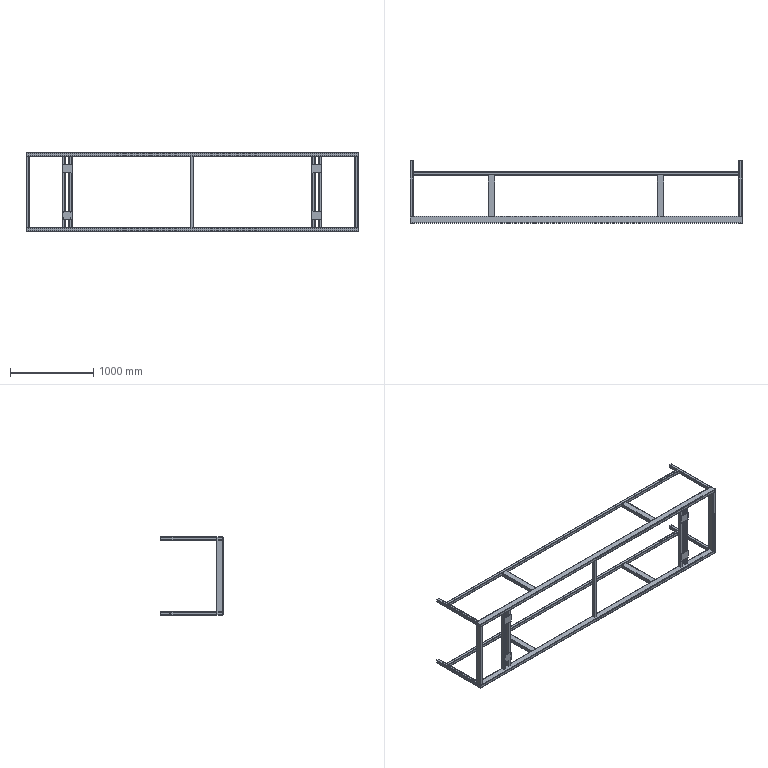Part | SolidWorks | features WeldCornerFeat 3, ICE 2, MirrorSolid 2, WeldMemberFeat 2, 3DProfileFeature 1, Cut 1, EndCap 1, Fillet 1, HoleWzd 1, MoveCopyBody 1, WeldmentFeature 1 | 27 solids | 426 faces | box 4000 x 750 x 940 mm | volume 14483541 mm3 | plane 242 | cylinder 184 | commonest cylinder face diameters 12 x84 6 x76 8.5 x16 10 x8